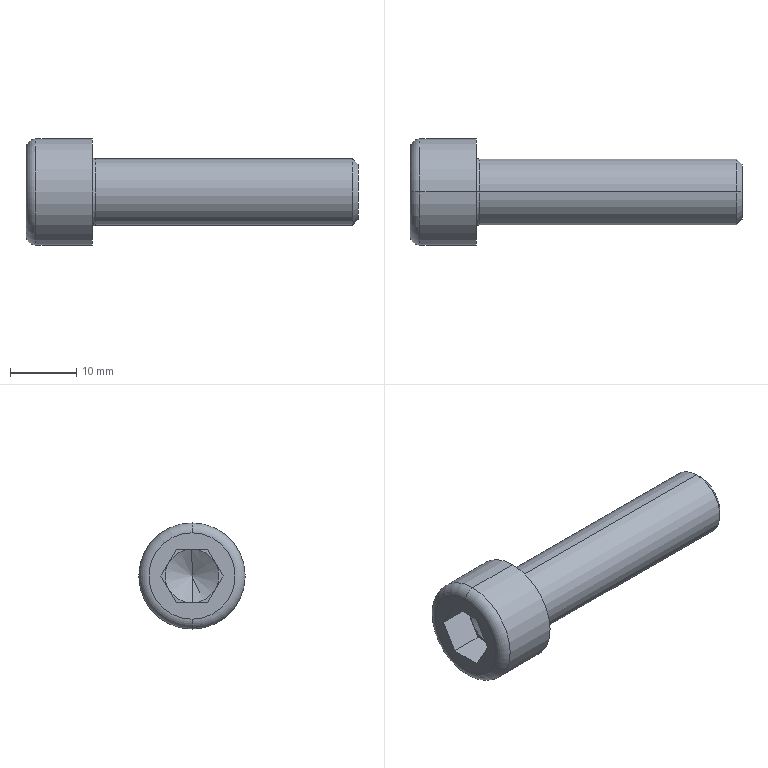Part | STEP file | socket head cap screw_iso(ISO 4762 M10 x 40 - 40N) | 1 solid | 27 faces | box 50 x 16 x 16 mm | volume 4794 mm3 | plane 15 | cone 4 | torus 4 | cylinder 4 | commonest cylinder face diameters 10 x2 16 x2